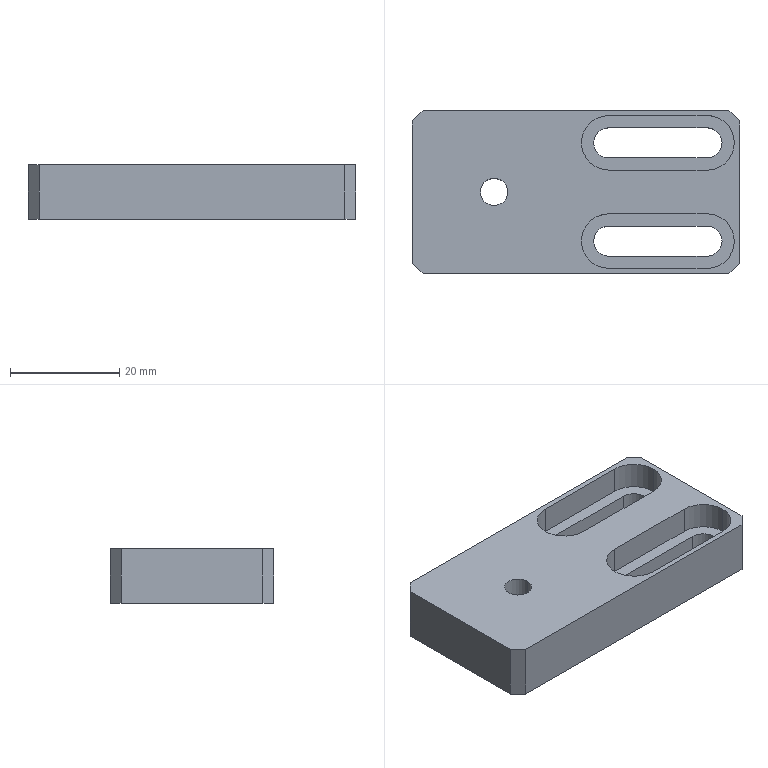Part | STEP file | 08-09 idler mounting plate | 1 solid | 34 faces | box 60 x 30 x 10 mm | volume 13911 mm3 | plane 20 | cylinder 14 | commonest cylinder face diameters 5.5 x6 10 x6 5 x2
STEP:
#1=CARTESIAN_POINT('',(29.,-9.,5.));
#2=VERTEX_POINT('',#1);
#3=CARTESIAN_POINT('',(24.,-4.,5.));
#4=VERTEX_POINT('',#3);
#5=CARTESIAN_POINT('',(24.,-9.,5.));
#6=DIRECTION('',(0.,0.,1.));
#7=DIRECTION('',(-1.,0.,0.));
#8=AXIS2_PLACEMENT_3D('',#5,#6,#7);
#9=CIRCLE('',#8,5.);
#10=EDGE_CURVE('',#2,#4,#9,.T.);
#11=ORIENTED_EDGE('',*,*,#10,.F.);
#12=CARTESIAN_POINT('',(29.,-9.,10.));
#13=VERTEX_POINT('',#12);
#14=CARTESIAN_POINT('',(29.,-9.,5.));
#15=DIRECTION('',(0.,0.,1.));
#16=VECTOR('',#15,1000.);
#17=LINE('',#14,#16);
#18=EDGE_CURVE('',#2,#13,#17,.T.);
#19=ORIENTED_EDGE('',*,*,#18,.T.);
#20=CARTESIAN_POINT('',(24.,-4.,10.));
#21=VERTEX_POINT('',#20);
#22=CARTESIAN_POINT('',(24.,-9.,10.));
#23=DIRECTION('',(0.,0.,1.));
#24=DIRECTION('',(-1.,0.,0.));
#25=AXIS2_PLACEMENT_3D('',#22,#23,#24);
#26=CIRCLE('',#25,5.);
#27=EDGE_CURVE('',#13,#21,#26,.T.);
#28=ORIENTED_EDGE('',*,*,#27,.T.);
#29=CARTESIAN_POINT('',(24.,-4.,5.));
#30=DIRECTION('',(0.,0.,1.));
#31=VECTOR('',#30,1000.);
#32=LINE('',#29,#31);
#33=EDGE_CURVE('',#4,#21,#32,.T.);
#34=ORIENTED_EDGE('',*,*,#33,.F.);
#35=EDGE_LOOP('',(#11,#19,#28,#34));
#36=FACE_OUTER_BOUND('',#35,.T.);
#37=CARTESIAN_POINT('',(24.,-9.,5.));
#38=DIRECTION('',(0.,0.,1.));
#39=DIRECTION('',(1.,0.,0.));
#40=AXIS2_PLACEMENT_3D('',#37,#38,#39);
#41=CYLINDRICAL_SURFACE('',#40,5.);
#42=ADVANCED_FACE('',(#36),#41,.F.);
#43=CARTESIAN_POINT('',(29.,9.,5.));
#44=VERTEX_POINT('',#43);
#45=CARTESIAN_POINT('',(24.,14.,5.));
#46=VERTEX_POINT('',#45);
#47=CARTESIAN_POINT('',(24.,9.,5.));
#48=DIRECTION('',(0.,0.,1.));
#49=DIRECTION('',(1.,0.,0.));
#50=AXIS2_PLACEMENT_3D('',#47,#48,#49);
#51=CIRCLE('',#50,5.);
#52=EDGE_CURVE('',#44,#46,#51,.T.);
#53=ORIENTED_EDGE('',*,*,#52,.F.);
#54=CARTESIAN_POINT('',(29.,9.,10.));
#55=VERTEX_POINT('',#54);
#56=CARTESIAN_POINT('',(29.,9.,5.));
#57=DIRECTION('',(0.,0.,1.));
#58=VECTOR('',#57,1000.);
#59=LINE('',#56,#58);
#60=EDGE_CURVE('',#44,#55,#59,.T.);
#61=ORIENTED_EDGE('',*,*,#60,.T.);
#62=CARTESIAN_POINT('',(24.,14.,10.));
#63=VERTEX_POINT('',#62);
#64=CARTESIAN_POINT('',(24.,9.,10.));
#65=DIRECTION('',(0.,0.,1.));
#66=DIRECTION('',(1.,0.,0.));
#67=AXIS2_PLACEMENT_3D('',#64,#65,#66);
#68=CIRCLE('',#67,5.);
#69=EDGE_CURVE('',#55,#63,#68,.T.);
#70=ORIENTED_EDGE('',*,*,#69,.T.);
#71=CARTESIAN_POINT('',(24.,14.,5.));
#72=DIRECTION('',(0.,0.,1.));
#73=VECTOR('',#72,1000.);
#74=LINE('',#71,#73);
#75=EDGE_CURVE('',#46,#63,#74,.T.);
#76=ORIENTED_EDGE('',*,*,#75,.F.);
#77=EDGE_LOOP('',(#53,#61,#70,#76));
#78=FACE_OUTER_BOUND('',#77,.T.);
#79=CARTESIAN_POINT('',(24.,9.,5.));
#80=DIRECTION('',(0.,0.,1.));
#81=DIRECTION('',(1.,0.,0.));
#82=AXIS2_PLACEMENT_3D('',#79,#80,#81);
#83=CYLINDRICAL_SURFACE('',#82,5.);
#84=ADVANCED_FACE('',(#78),#83,.F.);
#85=CARTESIAN_POINT('',(26.75,-9.,0.));
#86=VERTEX_POINT('',#85);
#87=CARTESIAN_POINT('',(24.,-6.25,0.));
#88=VERTEX_POINT('',#87);
#89=CARTESIAN_POINT('',(24.,-9.,0.));
#90=DIRECTION('',(0.,0.,1.));
#91=DIRECTION('',(-1.,0.,0.));
#92=AXIS2_PLACEMENT_3D('',#89,#90,#91);
#93=CIRCLE('',#92,2.75);
#94=EDGE_CURVE('',#86,#88,#93,.T.);
#95=ORIENTED_EDGE('',*,*,#94,.F.);
#96=CARTESIAN_POINT('',(26.75,-9.,5.));
#97=VERTEX_POINT('',#96);
#98=CARTESIAN_POINT('',(26.75,-9.,0.));
#99=DIRECTION('',(0.,0.,1.));
#100=VECTOR('',#99,1000.);
#101=LINE('',#98,#100);
#102=EDGE_CURVE('',#86,#97,#101,.T.);
#103=ORIENTED_EDGE('',*,*,#102,.T.);
#104=CARTESIAN_POINT('',(24.,-6.25,5.));
#105=VERTEX_POINT('',#104);
#106=CARTESIAN_POINT('',(24.,-9.,5.));
#107=DIRECTION('',(0.,0.,1.));
#108=DIRECTION('',(-1.,0.,0.));
#109=AXIS2_PLACEMENT_3D('',#106,#107,#108);
#110=CIRCLE('',#109,2.75);
#111=EDGE_CURVE('',#97,#105,#110,.T.);
#112=ORIENTED_EDGE('',*,*,#111,.T.);
#113=CARTESIAN_POINT('',(24.,-6.25,0.));
#114=DIRECTION('',(0.,0.,1.));
#115=VECTOR('',#114,1000.);
#116=LINE('',#113,#115);
#117=EDGE_CURVE('',#88,#105,#116,.T.);
#118=ORIENTED_EDGE('',*,*,#117,.F.);
#119=EDGE_LOOP('',(#95,#103,#112,#118));
#120=FACE_OUTER_BOUND('',#119,.T.);
#121=CARTESIAN_POINT('',(24.,-9.,0.));
#122=DIRECTION('',(0.,0.,1.));
#123=DIRECTION('',(1.,0.,0.));
#124=AXIS2_PLACEMENT_3D('',#121,#122,#123);
#125=CYLINDRICAL_SURFACE('',#124,2.75);
#126=ADVANCED_FACE('',(#120),#125,.F.);
#127=CARTESIAN_POINT('',(-17.5,0.,0.));
#128=VERTEX_POINT('',#127);
#129=CARTESIAN_POINT('',(-12.5,0.,0.));
#130=VERTEX_POINT('',#129);
#131=CARTESIAN_POINT('',(-15.,0.,0.));
#132=DIRECTION('',(0.,0.,1.));
#133=DIRECTION('',(1.,0.,0.));
#134=AXIS2_PLACEMENT_3D('',#131,#132,#133);
#135=CIRCLE('',#134,2.5);
#136=EDGE_CURVE('',#128,#130,#135,.T.);
#137=ORIENTED_EDGE('',*,*,#136,.F.);
#138=CARTESIAN_POINT('',(-17.5,0.,10.));
#139=VERTEX_POINT('',#138);
#140=CARTESIAN_POINT('',(-17.5,0.,10.));
#141=DIRECTION('',(0.,0.,1.));
#142=VECTOR('',#141,1000.);
#143=LINE('',#140,#142);
#144=EDGE_CURVE('',#128,#139,#143,.T.);
#145=ORIENTED_EDGE('',*,*,#144,.T.);
#146=CARTESIAN_POINT('',(-12.5,0.,10.));
#147=VERTEX_POINT('',#146);
#148=CARTESIAN_POINT('',(-15.,0.,10.));
#149=DIRECTION('',(0.,0.,1.));
#150=DIRECTION('',(1.,0.,0.));
#151=AXIS2_PLACEMENT_3D('',#148,#149,#150);
#152=CIRCLE('',#151,2.5);
#153=EDGE_CURVE('',#139,#147,#152,.T.);
#154=ORIENTED_EDGE('',*,*,#153,.T.);
#155=CARTESIAN_POINT('',(-12.5,0.,10.));
#156=DIRECTION('',(0.,0.,1.));
#157=VECTOR('',#156,1000.);
#158=LINE('',#155,#157);
#159=EDGE_CURVE('',#130,#147,#158,.T.);
#160=ORIENTED_EDGE('',*,*,#159,.F.);
#161=EDGE_LOOP('',(#137,#145,#154,#160));
#162=FACE_OUTER_BOUND('',#161,.T.);
#163=CARTESIAN_POINT('',(-15.,0.,10.));
#164=DIRECTION('',(0.,0.,1.));
#165=DIRECTION('',(1.,0.,0.));
#166=AXIS2_PLACEMENT_3D('',#163,#164,#165);
#167=CYLINDRICAL_SURFACE('',#166,2.5);
#168=ADVANCED_FACE('',(#162),#167,.F.);
#169=CARTESIAN_POINT('',(26.75,9.,0.));
#170=VERTEX_POINT('',#169);
#171=CARTESIAN_POINT('',(24.,11.75,0.));
#172=VERTEX_POINT('',#171);
#173=CARTESIAN_POINT('',(24.,9.,0.));
#174=DIRECTION('',(0.,0.,1.));
#175=DIRECTION('',(1.,0.,0.));
#176=AXIS2_PLACEMENT_3D('',#173,#174,#175);
#177=CIRCLE('',#176,2.75);
#178=EDGE_CURVE('',#170,#172,#177,.T.);
#179=ORIENTED_EDGE('',*,*,#178,.F.);
#180=CARTESIAN_POINT('',(26.75,9.,5.));
#181=VERTEX_POINT('',#180);
#182=CARTESIAN_POINT('',(26.75,9.,0.));
#183=DIRECTION('',(0.,0.,1.));
#184=VECTOR('',#183,1000.);
#185=LINE('',#182,#184);
#186=EDGE_CURVE('',#170,#181,#185,.T.);
#187=ORIENTED_EDGE('',*,*,#186,.T.);
#188=CARTESIAN_POINT('',(24.,11.75,5.));
#189=VERTEX_POINT('',#188);
#190=CARTESIAN_POINT('',(24.,9.,5.));
#191=DIRECTION('',(0.,0.,-1.));
#192=DIRECTION('',(1.,0.,0.));
#193=AXIS2_PLACEMENT_3D('',#190,#191,#192);
#194=CIRCLE('',#193,2.75);
#195=EDGE_CURVE('',#189,#181,#194,.T.);
#196=ORIENTED_EDGE('',*,*,#195,.F.);
#197=CARTESIAN_POINT('',(24.,11.75,0.));
#198=DIRECTION('',(0.,0.,1.));
#199=VECTOR('',#198,1000.);
#200=LINE('',#197,#199);
#201=EDGE_CURVE('',#172,#189,#200,.T.);
#202=ORIENTED_EDGE('',*,*,#201,.F.);
#203=EDGE_LOOP('',(#179,#187,#196,#202));
#204=FACE_OUTER_BOUND('',#203,.T.);
#205=CARTESIAN_POINT('',(24.,9.,0.));
#206=DIRECTION('',(0.,0.,1.));
#207=DIRECTION('',(1.,0.,0.));
#208=AXIS2_PLACEMENT_3D('',#205,#206,#207);
#209=CYLINDRICAL_SURFACE('',#208,2.75);
#210=ADVANCED_FACE('',(#204),#209,.F.);
#211=CARTESIAN_POINT('',(6.,6.25,5.));
#212=VERTEX_POINT('',#211);
#213=CARTESIAN_POINT('',(6.,11.75,5.));
#214=VERTEX_POINT('',#213);
#215=CARTESIAN_POINT('',(6.,9.,5.));
#216=DIRECTION('',(0.,0.,-1.));
#217=DIRECTION('',(1.,0.,0.));
#218=AXIS2_PLACEMENT_3D('',#215,#216,#217);
#219=CIRCLE('',#218,2.75);
#220=EDGE_CURVE('',#212,#214,#219,.T.);
#221=ORIENTED_EDGE('',*,*,#220,.F.);
#222=CARTESIAN_POINT('',(6.,6.25,0.));
#223=VERTEX_POINT('',#222);
#224=CARTESIAN_POINT('',(6.,6.25,0.));
#225=DIRECTION('',(0.,0.,1.));
#226=VECTOR('',#225,1000.);
#227=LINE('',#224,#226);
#228=EDGE_CURVE('',#223,#212,#227,.T.);
#229=ORIENTED_EDGE('',*,*,#228,.F.);
#230=CARTESIAN_POINT('',(6.,11.75,0.));
#231=VERTEX_POINT('',#230);
#232=CARTESIAN_POINT('',(6.,9.,0.));
#233=DIRECTION('',(0.,0.,1.));
#234=DIRECTION('',(1.,0.,0.));
#235=AXIS2_PLACEMENT_3D('',#232,#233,#234);
#236=CIRCLE('',#235,2.75);
#237=EDGE_CURVE('',#231,#223,#236,.T.);
#238=ORIENTED_EDGE('',*,*,#237,.F.);
#239=CARTESIAN_POINT('',(6.,11.75,0.));
#240=DIRECTION('',(0.,0.,1.));
#241=VECTOR('',#240,1000.);
#242=LINE('',#239,#241);
#243=EDGE_CURVE('',#231,#214,#242,.T.);
#244=ORIENTED_EDGE('',*,*,#243,.T.);
#245=EDGE_LOOP('',(#221,#229,#238,#244));
#246=FACE_OUTER_BOUND('',#245,.T.);
#247=CARTESIAN_POINT('',(6.,9.,0.));
#248=DIRECTION('',(0.,0.,1.));
#249=DIRECTION('',(1.,0.,0.));
#250=AXIS2_PLACEMENT_3D('',#247,#248,#249);
#251=CYLINDRICAL_SURFACE('',#250,2.75);
#252=ADVANCED_FACE('',(#246),#251,.F.);
#253=CARTESIAN_POINT('',(6.,11.75,5.));
#254=DIRECTION('',(1.,0.,0.));
#255=VECTOR('',#254,1000.);
#256=LINE('',#253,#255);
#257=EDGE_CURVE('',#214,#189,#256,.T.);
#258=ORIENTED_EDGE('',*,*,#257,.F.);
#259=ORIENTED_EDGE('',*,*,#243,.F.);
#260=CARTESIAN_POINT('',(6.,11.75,0.));
#261=DIRECTION('',(-1.,0.,0.));
#262=VECTOR('',#261,1000.);
#263=LINE('',#260,#262);
#264=EDGE_CURVE('',#172,#231,#263,.T.);
#265=ORIENTED_EDGE('',*,*,#264,.F.);
#266=ORIENTED_EDGE('',*,*,#201,.T.);
#267=EDGE_LOOP('',(#258,#259,#265,#266));
#268=FACE_OUTER_BOUND('',#267,.T.);
#269=CARTESIAN_POINT('',(6.,11.75,0.));
#270=DIRECTION('',(0.,1.,0.));
#271=DIRECTION('',(0.,0.,1.));
#272=AXIS2_PLACEMENT_3D('',#269,#270,#271);
#273=PLANE('',#272);
#274=ADVANCED_FACE('',(#268),#273,.F.);
#275=ORIENTED_EDGE('',*,*,#186,.F.);
#276=CARTESIAN_POINT('',(24.,6.25,0.));
#277=VERTEX_POINT('',#276);
#278=CARTESIAN_POINT('',(24.,9.,0.));
#279=DIRECTION('',(0.,0.,1.));
#280=DIRECTION('',(1.,0.,0.));
#281=AXIS2_PLACEMENT_3D('',#278,#279,#280);
#282=CIRCLE('',#281,2.75);
#283=EDGE_CURVE('',#277,#170,#282,.T.);
#284=ORIENTED_EDGE('',*,*,#283,.F.);
#285=CARTESIAN_POINT('',(24.,6.25,5.));
#286=VERTEX_POINT('',#285);
#287=CARTESIAN_POINT('',(24.,6.25,0.));
#288=DIRECTION('',(0.,0.,1.));
#289=VECTOR('',#288,1000.);
#290=LINE('',#287,#289);
#291=EDGE_CURVE('',#277,#286,#290,.T.);
#292=ORIENTED_EDGE('',*,*,#291,.T.);
#293=CARTESIAN_POINT('',(24.,9.,5.));
#294=DIRECTION('',(0.,0.,-1.));
#295=DIRECTION('',(1.,0.,0.));
#296=AXIS2_PLACEMENT_3D('',#293,#294,#295);
#297=CIRCLE('',#296,2.75);
#298=EDGE_CURVE('',#181,#286,#297,.T.);
#299=ORIENTED_EDGE('',*,*,#298,.F.);
#300=EDGE_LOOP('',(#275,#284,#292,#299));
#301=FACE_OUTER_BOUND('',#300,.T.);
#302=CARTESIAN_POINT('',(24.,9.,0.));
#303=DIRECTION('',(0.,0.,1.));
#304=DIRECTION('',(1.,0.,0.));
#305=AXIS2_PLACEMENT_3D('',#302,#303,#304);
#306=CYLINDRICAL_SURFACE('',#305,2.75);
#307=ADVANCED_FACE('',(#301),#306,.F.);
#308=CARTESIAN_POINT('',(6.,6.25,5.));
#309=DIRECTION('',(-1.,0.,0.));
#310=VECTOR('',#309,1000.);
#311=LINE('',#308,#310);
#312=EDGE_CURVE('',#286,#212,#311,.T.);
#313=ORIENTED_EDGE('',*,*,#312,.F.);
#314=ORIENTED_EDGE('',*,*,#291,.F.);
#315=CARTESIAN_POINT('',(6.,6.25,0.));
#316=DIRECTION('',(1.,0.,0.));
#317=VECTOR('',#316,1000.);
#318=LINE('',#315,#317);
#319=EDGE_CURVE('',#223,#277,#318,.T.);
#320=ORIENTED_EDGE('',*,*,#319,.F.);
#321=ORIENTED_EDGE('',*,*,#228,.T.);
#322=EDGE_LOOP('',(#313,#314,#320,#321));
#323=FACE_OUTER_BOUND('',#322,.T.);
#324=CARTESIAN_POINT('',(6.,6.25,0.));
#325=DIRECTION('',(0.,-1.,0.));
#326=DIRECTION('',(0.,0.,-1.));
#327=AXIS2_PLACEMENT_3D('',#324,#325,#326);
#328=PLANE('',#327);
#329=ADVANCED_FACE('',(#323),#328,.F.);
#330=CARTESIAN_POINT('',(30.,-13.,10.));
#331=VERTEX_POINT('',#330);
#332=CARTESIAN_POINT('',(30.,13.,10.));
#333=VERTEX_POINT('',#332);
#334=CARTESIAN_POINT('',(30.,15.,10.));
#335=DIRECTION('',(0.,1.,0.));
#336=VECTOR('',#335,1000.);
#337=LINE('',#334,#336);
#338=EDGE_CURVE('',#331,#333,#337,.T.);
#339=ORIENTED_EDGE('',*,*,#338,.F.);
#340=CARTESIAN_POINT('',(30.,-13.,0.));
#341=VERTEX_POINT('',#340);
#342=CARTESIAN_POINT('',(30.,-13.,10.));
#343=DIRECTION('',(0.,0.,-1.));
#344=VECTOR('',#343,1000.);
#345=LINE('',#342,#344);
#346=EDGE_CURVE('',#331,#341,#345,.T.);
#347=ORIENTED_EDGE('',*,*,#346,.T.);
#348=CARTESIAN_POINT('',(30.,13.,0.));
#349=VERTEX_POINT('',#348);
#350=CARTESIAN_POINT('',(30.,15.,0.));
#351=DIRECTION('',(0.,1.,0.));
#352=VECTOR('',#351,1000.);
#353=LINE('',#350,#352);
#354=EDGE_CURVE('',#341,#349,#353,.T.);
#355=ORIENTED_EDGE('',*,*,#354,.T.);
#356=CARTESIAN_POINT('',(30.,13.,10.));
#357=DIRECTION('',(0.,0.,1.));
#358=VECTOR('',#357,1000.);
#359=LINE('',#356,#358);
#360=EDGE_CURVE('',#349,#333,#359,.T.);
#361=ORIENTED_EDGE('',*,*,#360,.T.);
#362=EDGE_LOOP('',(#339,#347,#355,#361));
#363=FACE_OUTER_BOUND('',#362,.T.);
#364=CARTESIAN_POINT('',(30.,15.,10.));
#365=DIRECTION('',(-1.,0.,0.));
#366=DIRECTION('',(0.,-1.,0.));
#367=AXIS2_PLACEMENT_3D('',#364,#365,#366);
#368=PLANE('',#367);
#369=ADVANCED_FACE('',(#363),#368,.F.);
#370=CARTESIAN_POINT('',(28.,15.,10.));
#371=VERTEX_POINT('',#370);
#372=CARTESIAN_POINT('',(-28.,15.,10.));
#373=VERTEX_POINT('',#372);
#374=CARTESIAN_POINT('',(-30.,15.,10.));
#375=DIRECTION('',(-1.,0.,0.));
#376=VECTOR('',#375,1000.);
#377=LINE('',#374,#376);
#378=EDGE_CURVE('',#371,#373,#377,.T.);
#379=ORIENTED_EDGE('',*,*,#378,.F.);
#380=CARTESIAN_POINT('',(28.,15.,0.));
#381=VERTEX_POINT('',#380);
#382=CARTESIAN_POINT('',(28.,15.,10.));
#383=DIRECTION('',(0.,0.,-1.));
#384=VECTOR('',#383,1000.);
#385=LINE('',#382,#384);
#386=EDGE_CURVE('',#371,#381,#385,.T.);
#387=ORIENTED_EDGE('',*,*,#386,.T.);
#388=CARTESIAN_POINT('',(-28.,15.,0.));
#389=VERTEX_POINT('',#388);
#390=CARTESIAN_POINT('',(-30.,15.,0.));
#391=DIRECTION('',(-1.,0.,0.));
#392=VECTOR('',#391,1000.);
#393=LINE('',#390,#392);
#394=EDGE_CURVE('',#381,#389,#393,.T.);
#395=ORIENTED_EDGE('',*,*,#394,.T.);
#396=CARTESIAN_POINT('',(-28.,15.,10.));
#397=DIRECTION('',(0.,0.,1.));
#398=VECTOR('',#397,1000.);
#399=LINE('',#396,#398);
#400=EDGE_CURVE('',#389,#373,#399,.T.);
#401=ORIENTED_EDGE('',*,*,#400,.T.);
#402=EDGE_LOOP('',(#379,#387,#395,#401));
#403=FACE_OUTER_BOUND('',#402,.T.);
#404=CARTESIAN_POINT('',(-30.,15.,10.));
#405=DIRECTION('',(0.,-1.,0.));
#406=DIRECTION('',(0.,0.,-1.));
#407=AXIS2_PLACEMENT_3D('',#404,#405,#406);
#408=PLANE('',#407);
#409=ADVANCED_FACE('',(#403),#408,.F.);
#410=CARTESIAN_POINT('',(-30.,13.,0.));
#411=VERTEX_POINT('',#410);
#412=CARTESIAN_POINT('',(-30.,-13.,0.));
#413=VERTEX_POINT('',#412);
#414=CARTESIAN_POINT('',(-30.,15.,0.));
#415=DIRECTION('',(0.,-1.,0.));
#416=VECTOR('',#415,1000.);
#417=LINE('',#414,#416);
#418=EDGE_CURVE('',#411,#413,#417,.T.);
#419=ORIENTED_EDGE('',*,*,#418,.T.);
#420=CARTESIAN_POINT('',(-30.,-13.,10.));
#421=VERTEX_POINT('',#420);
#422=CARTESIAN_POINT('',(-30.,-13.,10.));
#423=DIRECTION('',(0.,0.,1.));
#424=VECTOR('',#423,1000.);
#425=LINE('',#422,#424);
#426=EDGE_CURVE('',#413,#421,#425,.T.);
#427=ORIENTED_EDGE('',*,*,#426,.T.);
#428=CARTESIAN_POINT('',(-30.,13.,10.));
#429=VERTEX_POINT('',#428);
#430=CARTESIAN_POINT('',(-30.,15.,10.));
#431=DIRECTION('',(0.,-1.,0.));
#432=VECTOR('',#431,1000.);
#433=LINE('',#430,#432);
#434=EDGE_CURVE('',#429,#421,#433,.T.);
#435=ORIENTED_EDGE('',*,*,#434,.F.);
#436=CARTESIAN_POINT('',(-30.,13.,10.));
#437=DIRECTION('',(0.,0.,-1.));
#438=VECTOR('',#437,1000.);
#439=LINE('',#436,#438);
#440=EDGE_CURVE('',#429,#411,#439,.T.);
#441=ORIENTED_EDGE('',*,*,#440,.T.);
#442=EDGE_LOOP('',(#419,#427,#435,#441));
#443=FACE_OUTER_BOUND('',#442,.T.);
#444=CARTESIAN_POINT('',(-30.,15.,10.));
#445=DIRECTION('',(1.,0.,0.));
#446=DIRECTION('',(0.,1.,0.));
#447=AXIS2_PLACEMENT_3D('',#444,#445,#446);
#448=PLANE('',#447);
#449=ADVANCED_FACE('',(#443),#448,.F.);
#450=CARTESIAN_POINT('',(-28.,-15.,0.));
#451=VERTEX_POINT('',#450);
#452=CARTESIAN_POINT('',(28.,-15.,0.));
#453=VERTEX_POINT('',#452);
#454=CARTESIAN_POINT('',(-30.,-15.,0.));
#455=DIRECTION('',(1.,0.,0.));
#456=VECTOR('',#455,1000.);
#457=LINE('',#454,#456);
#458=EDGE_CURVE('',#451,#453,#457,.T.);
#459=ORIENTED_EDGE('',*,*,#458,.T.);
#460=CARTESIAN_POINT('',(28.,-15.,10.));
#461=VERTEX_POINT('',#460);
#462=CARTESIAN_POINT('',(28.,-15.,10.));
#463=DIRECTION('',(0.,0.,1.));
#464=VECTOR('',#463,1000.);
#465=LINE('',#462,#464);
#466=EDGE_CURVE('',#453,#461,#465,.T.);
#467=ORIENTED_EDGE('',*,*,#466,.T.);
#468=CARTESIAN_POINT('',(-28.,-15.,10.));
#469=VERTEX_POINT('',#468);
#470=CARTESIAN_POINT('',(-30.,-15.,10.));
#471=DIRECTION('',(1.,0.,0.));
#472=VECTOR('',#471,1000.);
#473=LINE('',#470,#472);
#474=EDGE_CURVE('',#469,#461,#473,.T.);
#475=ORIENTED_EDGE('',*,*,#474,.F.);
#476=CARTESIAN_POINT('',(-28.,-15.,10.));
#477=DIRECTION('',(0.,0.,-1.));
#478=VECTOR('',#477,1000.);
#479=LINE('',#476,#478);
#480=EDGE_CURVE('',#469,#451,#479,.T.);
#481=ORIENTED_EDGE('',*,*,#480,.T.);
#482=EDGE_LOOP('',(#459,#467,#475,#481));
#483=FACE_OUTER_BOUND('',#482,.T.);
#484=CARTESIAN_POINT('',(-30.,-15.,10.));
#485=DIRECTION('',(0.,1.,0.));
#486=DIRECTION('',(0.,0.,1.));
#487=AXIS2_PLACEMENT_3D('',#484,#485,#486);
#488=PLANE('',#487);
#489=ADVANCED_FACE('',(#483),#488,.F.);
#490=CARTESIAN_POINT('',(6.,-4.,10.));
#491=VERTEX_POINT('',#490);
#492=CARTESIAN_POINT('',(6.,-14.,10.));
#493=VERTEX_POINT('',#492);
#494=CARTESIAN_POINT('',(6.,-9.,10.));
#495=DIRECTION('',(0.,0.,1.));
#496=DIRECTION('',(-1.,0.,0.));
#497=AXIS2_PLACEMENT_3D('',#494,#495,#496);
#498=CIRCLE('',#497,5.);
#499=EDGE_CURVE('',#491,#493,#498,.T.);
#500=ORIENTED_EDGE('',*,*,#499,.F.);
#501=CARTESIAN_POINT('',(6.,-4.,10.));
#502=DIRECTION('',(-1.,0.,0.));
#503=VECTOR('',#502,1000.);
#504=LINE('',#501,#503);
#505=EDGE_CURVE('',#21,#491,#504,.T.);
#506=ORIENTED_EDGE('',*,*,#505,.F.);
#507=ORIENTED_EDGE('',*,*,#27,.F.);
#508=CARTESIAN_POINT('',(24.,-14.,10.));
#509=VERTEX_POINT('',#508);
#510=CARTESIAN_POINT('',(24.,-9.,10.));
#511=DIRECTION('',(0.,0.,1.));
#512=DIRECTION('',(-1.,0.,0.));
#513=AXIS2_PLACEMENT_3D('',#510,#511,#512);
#514=CIRCLE('',#513,5.);
#515=EDGE_CURVE('',#509,#13,#514,.T.);
#516=ORIENTED_EDGE('',*,*,#515,.F.);
#517=CARTESIAN_POINT('',(6.,-14.,10.));
#518=DIRECTION('',(1.,0.,0.));
#519=VECTOR('',#518,1000.);
#520=LINE('',#517,#519);
#521=EDGE_CURVE('',#493,#509,#520,.T.);
#522=ORIENTED_EDGE('',*,*,#521,.F.);
#523=EDGE_LOOP('',(#500,#506,#507,#516,#522));
#524=FACE_BOUND('',#523,.T.);
#525=CARTESIAN_POINT('',(6.,14.,10.));
#526=VERTEX_POINT('',#525);
#527=CARTESIAN_POINT('',(6.,4.,10.));
#528=VERTEX_POINT('',#527);
#529=CARTESIAN_POINT('',(6.,9.,10.));
#530=DIRECTION('',(0.,0.,1.));
#531=DIRECTION('',(1.,0.,0.));
#532=AXIS2_PLACEMENT_3D('',#529,#530,#531);
#533=CIRCLE('',#532,5.);
#534=EDGE_CURVE('',#526,#528,#533,.T.);
#535=ORIENTED_EDGE('',*,*,#534,.F.);
#536=CARTESIAN_POINT('',(6.,14.,10.));
#537=DIRECTION('',(-1.,0.,0.));
#538=VECTOR('',#537,1000.);
#539=LINE('',#536,#538);
#540=EDGE_CURVE('',#63,#526,#539,.T.);
#541=ORIENTED_EDGE('',*,*,#540,.F.);
#542=ORIENTED_EDGE('',*,*,#69,.F.);
#543=CARTESIAN_POINT('',(24.,4.,10.));
#544=VERTEX_POINT('',#543);
#545=CARTESIAN_POINT('',(24.,9.,10.));
#546=DIRECTION('',(0.,0.,1.));
#547=DIRECTION('',(1.,0.,0.));
#548=AXIS2_PLACEMENT_3D('',#545,#546,#547);
#549=CIRCLE('',#548,5.);
#550=EDGE_CURVE('',#544,#55,#549,.T.);
#551=ORIENTED_EDGE('',*,*,#550,.F.);
#552=CARTESIAN_POINT('',(6.,4.,10.));
#553=DIRECTION('',(1.,0.,0.));
#554=VECTOR('',#553,1000.);
#555=LINE('',#552,#554);
#556=EDGE_CURVE('',#528,#544,#555,.T.);
#557=ORIENTED_EDGE('',*,*,#556,.F.);
#558=EDGE_LOOP('',(#535,#541,#542,#551,#557));
#559=FACE_BOUND('',#558,.T.);
#560=CARTESIAN_POINT('',(-15.,0.,10.));
#561=DIRECTION('',(0.,0.,1.));
#562=DIRECTION('',(1.,0.,0.));
#563=AXIS2_PLACEMENT_3D('',#560,#561,#562);
#564=CIRCLE('',#563,2.5);
#565=EDGE_CURVE('',#147,#139,#564,.T.);
#566=ORIENTED_EDGE('',*,*,#565,.F.);
#567=ORIENTED_EDGE('',*,*,#153,.F.);
#568=EDGE_LOOP('',(#566,#567));
#569=FACE_BOUND('',#568,.T.);
#570=ORIENTED_EDGE('',*,*,#474,.T.);
#571=CARTESIAN_POINT('',(29.,-14.,10.));
#572=DIRECTION('',(0.7071,0.7071,0.));
#573=VECTOR('',#572,1000.);
#574=LINE('',#571,#573);
#575=EDGE_CURVE('',#461,#331,#574,.T.);
#576=ORIENTED_EDGE('',*,*,#575,.T.);
#577=ORIENTED_EDGE('',*,*,#338,.T.);
#578=CARTESIAN_POINT('',(44.,-1.,10.));
#579=DIRECTION('',(-0.7071,0.7071,0.));
#580=VECTOR('',#579,1000.);
#581=LINE('',#578,#580);
#582=EDGE_CURVE('',#333,#371,#581,.T.);
#583=ORIENTED_EDGE('',*,*,#582,.T.);
#584=ORIENTED_EDGE('',*,*,#378,.T.);
#585=CARTESIAN_POINT('',(-14.,29.,10.));
#586=DIRECTION('',(-0.7071,-0.7071,0.));
#587=VECTOR('',#586,1000.);
#588=LINE('',#585,#587);
#589=EDGE_CURVE('',#373,#429,#588,.T.);
#590=ORIENTED_EDGE('',*,*,#589,.T.);
#591=ORIENTED_EDGE('',*,*,#434,.T.);
#592=CARTESIAN_POINT('',(1.,-44.,10.));
#593=DIRECTION('',(0.7071,-0.7071,0.));
#594=VECTOR('',#593,1000.);
#595=LINE('',#592,#594);
#596=EDGE_CURVE('',#421,#469,#595,.T.);
#597=ORIENTED_EDGE('',*,*,#596,.T.);
#598=EDGE_LOOP('',(#570,#576,#577,#583,#584,#590,#591,#597));
#599=FACE_OUTER_BOUND('',#598,.T.);
#600=CARTESIAN_POINT('',(30.,-15.,10.));
#601=DIRECTION('',(0.,0.,1.));
#602=DIRECTION('',(1.,0.,0.));
#603=AXIS2_PLACEMENT_3D('',#600,#601,#602);
#604=PLANE('',#603);
#605=ADVANCED_FACE('',(#524,#559,#569,#599),#604,.T.);
#606=CARTESIAN_POINT('',(6.,-6.25,0.));
#607=VERTEX_POINT('',#606);
#608=CARTESIAN_POINT('',(6.,-6.25,0.));
#609=DIRECTION('',(-1.,0.,0.));
#610=VECTOR('',#609,1000.);
#611=LINE('',#608,#610);
#612=EDGE_CURVE('',#88,#607,#611,.T.);
#613=ORIENTED_EDGE('',*,*,#612,.T.);
#614=CARTESIAN_POINT('',(6.,-11.75,0.));
#615=VERTEX_POINT('',#614);
#616=CARTESIAN_POINT('',(6.,-9.,0.));
#617=DIRECTION('',(0.,0.,1.));
#618=DIRECTION('',(-1.,0.,0.));
#619=AXIS2_PLACEMENT_3D('',#616,#617,#618);
#620=CIRCLE('',#619,2.75);
#621=EDGE_CURVE('',#607,#615,#620,.T.);
#622=ORIENTED_EDGE('',*,*,#621,.T.);
#623=CARTESIAN_POINT('',(24.,-11.75,0.));
#624=VERTEX_POINT('',#623);
#625=CARTESIAN_POINT('',(6.,-11.75,0.));
#626=DIRECTION('',(1.,0.,0.));
#627=VECTOR('',#626,1000.);
#628=LINE('',#625,#627);
#629=EDGE_CURVE('',#615,#624,#628,.T.);
#630=ORIENTED_EDGE('',*,*,#629,.T.);
#631=CARTESIAN_POINT('',(24.,-9.,0.));
#632=DIRECTION('',(0.,0.,1.));
#633=DIRECTION('',(-1.,0.,0.));
#634=AXIS2_PLACEMENT_3D('',#631,#632,#633);
#635=CIRCLE('',#634,2.75);
#636=EDGE_CURVE('',#624,#86,#635,.T.);
#637=ORIENTED_EDGE('',*,*,#636,.T.);
#638=ORIENTED_EDGE('',*,*,#94,.T.);
#639=EDGE_LOOP('',(#613,#622,#630,#637,#638));
#640=FACE_BOUND('',#639,.T.);
#641=ORIENTED_EDGE('',*,*,#264,.T.);
#642=ORIENTED_EDGE('',*,*,#237,.T.);
#643=ORIENTED_EDGE('',*,*,#319,.T.);
#644=ORIENTED_EDGE('',*,*,#283,.T.);
#645=ORIENTED_EDGE('',*,*,#178,.T.);
#646=EDGE_LOOP('',(#641,#642,#643,#644,#645));
#647=FACE_BOUND('',#646,.T.);
#648=CARTESIAN_POINT('',(-15.,0.,0.));
#649=DIRECTION('',(0.,0.,1.));
#650=DIRECTION('',(1.,0.,0.));
#651=AXIS2_PLACEMENT_3D('',#648,#649,#650);
#652=CIRCLE('',#651,2.5);
#653=EDGE_CURVE('',#130,#128,#652,.T.);
#654=ORIENTED_EDGE('',*,*,#653,.T.);
#655=ORIENTED_EDGE('',*,*,#136,.T.);
#656=EDGE_LOOP('',(#654,#655));
#657=FACE_BOUND('',#656,.T.);
#658=ORIENTED_EDGE('',*,*,#354,.F.);
#659=CARTESIAN_POINT('',(30.,-13.,0.));
#660=DIRECTION('',(-0.7071,-0.7071,0.));
#661=VECTOR('',#660,1000.);
#662=LINE('',#659,#661);
#663=EDGE_CURVE('',#341,#453,#662,.T.);
#664=ORIENTED_EDGE('',*,*,#663,.T.);
#665=ORIENTED_EDGE('',*,*,#458,.F.);
#666=CARTESIAN_POINT('',(-28.,-15.,0.));
#667=DIRECTION('',(-0.7071,0.7071,0.));
#668=VECTOR('',#667,1000.);
#669=LINE('',#666,#668);
#670=EDGE_CURVE('',#451,#413,#669,.T.);
#671=ORIENTED_EDGE('',*,*,#670,.T.);
#672=ORIENTED_EDGE('',*,*,#418,.F.);
#673=CARTESIAN_POINT('',(-30.,13.,0.));
#674=DIRECTION('',(0.7071,0.7071,0.));
#675=VECTOR('',#674,1000.);
#676=LINE('',#673,#675);
#677=EDGE_CURVE('',#411,#389,#676,.T.);
#678=ORIENTED_EDGE('',*,*,#677,.T.);
#679=ORIENTED_EDGE('',*,*,#394,.F.);
#680=CARTESIAN_POINT('',(28.,15.,0.));
#681=DIRECTION('',(0.7071,-0.7071,0.));
#682=VECTOR('',#681,1000.);
#683=LINE('',#680,#682);
#684=EDGE_CURVE('',#381,#349,#683,.T.);
#685=ORIENTED_EDGE('',*,*,#684,.T.);
#686=EDGE_LOOP('',(#658,#664,#665,#671,#672,#678,#679,#685));
#687=FACE_OUTER_BOUND('',#686,.T.);
#688=CARTESIAN_POINT('',(30.,-15.,0.));
#689=DIRECTION('',(0.,0.,1.));
#690=DIRECTION('',(1.,0.,0.));
#691=AXIS2_PLACEMENT_3D('',#688,#689,#690);
#692=PLANE('',#691);
#693=ADVANCED_FACE('',(#640,#647,#657,#687),#692,.F.);
#694=ORIENTED_EDGE('',*,*,#144,.F.);
#695=ORIENTED_EDGE('',*,*,#653,.F.);
#696=ORIENTED_EDGE('',*,*,#159,.T.);
#697=ORIENTED_EDGE('',*,*,#565,.T.);
#698=EDGE_LOOP('',(#694,#695,#696,#697));
#699=FACE_OUTER_BOUND('',#698,.T.);
#700=CARTESIAN_POINT('',(-15.,0.,10.));
#701=DIRECTION('',(0.,0.,1.));
#702=DIRECTION('',(1.,0.,0.));
#703=AXIS2_PLACEMENT_3D('',#700,#701,#702);
#704=CYLINDRICAL_SURFACE('',#703,2.5);
#705=ADVANCED_FACE('',(#699),#704,.F.);
#706=ORIENTED_EDGE('',*,*,#575,.F.);
#707=ORIENTED_EDGE('',*,*,#466,.F.);
#708=ORIENTED_EDGE('',*,*,#663,.F.);
#709=ORIENTED_EDGE('',*,*,#346,.F.);
#710=EDGE_LOOP('',(#706,#707,#708,#709));
#711=FACE_OUTER_BOUND('',#710,.T.);
#712=CARTESIAN_POINT('',(30.,-13.,10.));
#713=DIRECTION('',(-0.7071,0.7071,0.));
#714=DIRECTION('',(-0.7071,-0.7071,0.));
#715=AXIS2_PLACEMENT_3D('',#712,#713,#714);
#716=PLANE('',#715);
#717=ADVANCED_FACE('',(#711),#716,.F.);
#718=ORIENTED_EDGE('',*,*,#582,.F.);
#719=ORIENTED_EDGE('',*,*,#360,.F.);
#720=ORIENTED_EDGE('',*,*,#684,.F.);
#721=ORIENTED_EDGE('',*,*,#386,.F.);
#722=EDGE_LOOP('',(#718,#719,#720,#721));
#723=FACE_OUTER_BOUND('',#722,.T.);
#724=CARTESIAN_POINT('',(28.,15.,10.));
#725=DIRECTION('',(-0.7071,-0.7071,0.));
#726=DIRECTION('',(0.7071,-0.7071,0.));
#727=AXIS2_PLACEMENT_3D('',#724,#725,#726);
#728=PLANE('',#727);
#729=ADVANCED_FACE('',(#723),#728,.F.);
#730=ORIENTED_EDGE('',*,*,#596,.F.);
#731=ORIENTED_EDGE('',*,*,#426,.F.);
#732=ORIENTED_EDGE('',*,*,#670,.F.);
#733=ORIENTED_EDGE('',*,*,#480,.F.);
#734=EDGE_LOOP('',(#730,#731,#732,#733));
#735=FACE_OUTER_BOUND('',#734,.T.);
#736=CARTESIAN_POINT('',(-28.,-15.,10.));
#737=DIRECTION('',(0.7071,0.7071,0.));
#738=DIRECTION('',(-0.7071,0.7071,0.));
#739=AXIS2_PLACEMENT_3D('',#736,#737,#738);
#740=PLANE('',#739);
#741=ADVANCED_FACE('',(#735),#740,.F.);
#742=ORIENTED_EDGE('',*,*,#589,.F.);
#743=ORIENTED_EDGE('',*,*,#400,.F.);
#744=ORIENTED_EDGE('',*,*,#677,.F.);
#745=ORIENTED_EDGE('',*,*,#440,.F.);
#746=EDGE_LOOP('',(#742,#743,#744,#745));
#747=FACE_OUTER_BOUND('',#746,.T.);
#748=CARTESIAN_POINT('',(-30.,13.,10.));
#749=DIRECTION('',(0.7071,-0.7071,0.));
#750=DIRECTION('',(0.7071,0.7071,0.));
#751=AXIS2_PLACEMENT_3D('',#748,#749,#750);
#752=PLANE('',#751);
#753=ADVANCED_FACE('',(#747),#752,.F.);
#754=CARTESIAN_POINT('',(6.,-6.25,5.));
#755=VERTEX_POINT('',#754);
#756=CARTESIAN_POINT('',(6.,-6.25,0.));
#757=DIRECTION('',(0.,0.,1.));
#758=VECTOR('',#757,1000.);
#759=LINE('',#756,#758);
#760=EDGE_CURVE('',#607,#755,#759,.T.);
#761=ORIENTED_EDGE('',*,*,#760,.T.);
#762=CARTESIAN_POINT('',(6.,-11.75,5.));
#763=VERTEX_POINT('',#762);
#764=CARTESIAN_POINT('',(6.,-9.,5.));
#765=DIRECTION('',(0.,0.,1.));
#766=DIRECTION('',(-1.,0.,0.));
#767=AXIS2_PLACEMENT_3D('',#764,#765,#766);
#768=CIRCLE('',#767,2.75);
#769=EDGE_CURVE('',#755,#763,#768,.T.);
#770=ORIENTED_EDGE('',*,*,#769,.T.);
#771=CARTESIAN_POINT('',(6.,-11.75,0.));
#772=DIRECTION('',(0.,0.,1.));
#773=VECTOR('',#772,1000.);
#774=LINE('',#771,#773);
#775=EDGE_CURVE('',#615,#763,#774,.T.);
#776=ORIENTED_EDGE('',*,*,#775,.F.);
#777=ORIENTED_EDGE('',*,*,#621,.F.);
#778=EDGE_LOOP('',(#761,#770,#776,#777));
#779=FACE_OUTER_BOUND('',#778,.T.);
#780=CARTESIAN_POINT('',(6.,-9.,0.));
#781=DIRECTION('',(0.,0.,1.));
#782=DIRECTION('',(1.,0.,0.));
#783=AXIS2_PLACEMENT_3D('',#780,#781,#782);
#784=CYLINDRICAL_SURFACE('',#783,2.75);
#785=ADVANCED_FACE('',(#779),#784,.F.);
#786=ORIENTED_EDGE('',*,*,#117,.T.);
#787=CARTESIAN_POINT('',(6.,-6.25,5.));
#788=DIRECTION('',(-1.,0.,0.));
#789=VECTOR('',#788,1000.);
#790=LINE('',#787,#789);
#791=EDGE_CURVE('',#105,#755,#790,.T.);
#792=ORIENTED_EDGE('',*,*,#791,.T.);
#793=ORIENTED_EDGE('',*,*,#760,.F.);
#794=ORIENTED_EDGE('',*,*,#612,.F.);
#795=EDGE_LOOP('',(#786,#792,#793,#794));
#796=FACE_OUTER_BOUND('',#795,.T.);
#797=CARTESIAN_POINT('',(6.,-6.25,0.));
#798=DIRECTION('',(0.,1.,0.));
#799=DIRECTION('',(0.,0.,1.));
#800=AXIS2_PLACEMENT_3D('',#797,#798,#799);
#801=PLANE('',#800);
#802=ADVANCED_FACE('',(#796),#801,.F.);
#803=ORIENTED_EDGE('',*,*,#102,.F.);
#804=ORIENTED_EDGE('',*,*,#636,.F.);
#805=CARTESIAN_POINT('',(24.,-11.75,5.));
#806=VERTEX_POINT('',#805);
#807=CARTESIAN_POINT('',(24.,-11.75,0.));
#808=DIRECTION('',(0.,0.,1.));
#809=VECTOR('',#808,1000.);
#810=LINE('',#807,#809);
#811=EDGE_CURVE('',#624,#806,#810,.T.);
#812=ORIENTED_EDGE('',*,*,#811,.T.);
#813=CARTESIAN_POINT('',(24.,-9.,5.));
#814=DIRECTION('',(0.,0.,1.));
#815=DIRECTION('',(-1.,0.,0.));
#816=AXIS2_PLACEMENT_3D('',#813,#814,#815);
#817=CIRCLE('',#816,2.75);
#818=EDGE_CURVE('',#806,#97,#817,.T.);
#819=ORIENTED_EDGE('',*,*,#818,.T.);
#820=EDGE_LOOP('',(#803,#804,#812,#819));
#821=FACE_OUTER_BOUND('',#820,.T.);
#822=CARTESIAN_POINT('',(24.,-9.,0.));
#823=DIRECTION('',(0.,0.,1.));
#824=DIRECTION('',(1.,0.,0.));
#825=AXIS2_PLACEMENT_3D('',#822,#823,#824);
#826=CYLINDRICAL_SURFACE('',#825,2.75);
#827=ADVANCED_FACE('',(#821),#826,.F.);
#828=ORIENTED_EDGE('',*,*,#775,.T.);
#829=CARTESIAN_POINT('',(6.,-11.75,5.));
#830=DIRECTION('',(1.,0.,0.));
#831=VECTOR('',#830,1000.);
#832=LINE('',#829,#831);
#833=EDGE_CURVE('',#763,#806,#832,.T.);
#834=ORIENTED_EDGE('',*,*,#833,.T.);
#835=ORIENTED_EDGE('',*,*,#811,.F.);
#836=ORIENTED_EDGE('',*,*,#629,.F.);
#837=EDGE_LOOP('',(#828,#834,#835,#836));
#838=FACE_OUTER_BOUND('',#837,.T.);
#839=CARTESIAN_POINT('',(6.,-11.75,0.));
#840=DIRECTION('',(0.,-1.,0.));
#841=DIRECTION('',(0.,0.,-1.));
#842=AXIS2_PLACEMENT_3D('',#839,#840,#841);
#843=PLANE('',#842);
#844=ADVANCED_FACE('',(#838),#843,.F.);
#845=CARTESIAN_POINT('',(6.,14.,5.));
#846=VERTEX_POINT('',#845);
#847=CARTESIAN_POINT('',(6.,4.,5.));
#848=VERTEX_POINT('',#847);
#849=CARTESIAN_POINT('',(6.,9.,5.));
#850=DIRECTION('',(0.,0.,1.));
#851=DIRECTION('',(1.,0.,0.));
#852=AXIS2_PLACEMENT_3D('',#849,#850,#851);
#853=CIRCLE('',#852,5.);
#854=EDGE_CURVE('',#846,#848,#853,.T.);
#855=ORIENTED_EDGE('',*,*,#854,.T.);
#856=CARTESIAN_POINT('',(24.,4.,5.));
#857=VERTEX_POINT('',#856);
#858=CARTESIAN_POINT('',(6.,4.,5.));
#859=DIRECTION('',(1.,0.,0.));
#860=VECTOR('',#859,1000.);
#861=LINE('',#858,#860);
#862=EDGE_CURVE('',#848,#857,#861,.T.);
#863=ORIENTED_EDGE('',*,*,#862,.T.);
#864=CARTESIAN_POINT('',(24.,9.,5.));
#865=DIRECTION('',(0.,0.,1.));
#866=DIRECTION('',(1.,0.,0.));
#867=AXIS2_PLACEMENT_3D('',#864,#865,#866);
#868=CIRCLE('',#867,5.);
#869=EDGE_CURVE('',#857,#44,#868,.T.);
#870=ORIENTED_EDGE('',*,*,#869,.T.);
#871=ORIENTED_EDGE('',*,*,#52,.T.);
#872=CARTESIAN_POINT('',(6.,14.,5.));
#873=DIRECTION('',(-1.,0.,0.));
#874=VECTOR('',#873,1000.);
#875=LINE('',#872,#874);
#876=EDGE_CURVE('',#46,#846,#875,.T.);
#877=ORIENTED_EDGE('',*,*,#876,.T.);
#878=EDGE_LOOP('',(#855,#863,#870,#871,#877));
#879=FACE_OUTER_BOUND('',#878,.T.);
#880=ORIENTED_EDGE('',*,*,#220,.T.);
#881=ORIENTED_EDGE('',*,*,#257,.T.);
#882=ORIENTED_EDGE('',*,*,#195,.T.);
#883=ORIENTED_EDGE('',*,*,#298,.T.);
#884=ORIENTED_EDGE('',*,*,#312,.T.);
#885=EDGE_LOOP('',(#880,#881,#882,#883,#884));
#886=FACE_BOUND('',#885,.T.);
#887=CARTESIAN_POINT('',(6.,9.,5.));
#888=DIRECTION('',(0.,0.,1.));
#889=DIRECTION('',(1.,0.,0.));
#890=AXIS2_PLACEMENT_3D('',#887,#888,#889);
#891=PLANE('',#890);
#892=ADVANCED_FACE('',(#879,#886),#891,.T.);
#893=ORIENTED_EDGE('',*,*,#534,.T.);
#894=CARTESIAN_POINT('',(6.,4.,5.));
#895=DIRECTION('',(0.,0.,1.));
#896=VECTOR('',#895,1000.);
#897=LINE('',#894,#896);
#898=EDGE_CURVE('',#848,#528,#897,.T.);
#899=ORIENTED_EDGE('',*,*,#898,.F.);
#900=ORIENTED_EDGE('',*,*,#854,.F.);
#901=CARTESIAN_POINT('',(6.,14.,5.));
#902=DIRECTION('',(0.,0.,1.));
#903=VECTOR('',#902,1000.);
#904=LINE('',#901,#903);
#905=EDGE_CURVE('',#846,#526,#904,.T.);
#906=ORIENTED_EDGE('',*,*,#905,.T.);
#907=EDGE_LOOP('',(#893,#899,#900,#906));
#908=FACE_OUTER_BOUND('',#907,.T.);
#909=CARTESIAN_POINT('',(6.,9.,5.));
#910=DIRECTION('',(0.,0.,1.));
#911=DIRECTION('',(1.,0.,0.));
#912=AXIS2_PLACEMENT_3D('',#909,#910,#911);
#913=CYLINDRICAL_SURFACE('',#912,5.);
#914=ADVANCED_FACE('',(#908),#913,.F.);
#915=ORIENTED_EDGE('',*,*,#540,.T.);
#916=ORIENTED_EDGE('',*,*,#905,.F.);
#917=ORIENTED_EDGE('',*,*,#876,.F.);
#918=ORIENTED_EDGE('',*,*,#75,.T.);
#919=EDGE_LOOP('',(#915,#916,#917,#918));
#920=FACE_OUTER_BOUND('',#919,.T.);
#921=CARTESIAN_POINT('',(6.,14.,5.));
#922=DIRECTION('',(0.,1.,0.));
#923=DIRECTION('',(0.,0.,1.));
#924=AXIS2_PLACEMENT_3D('',#921,#922,#923);
#925=PLANE('',#924);
#926=ADVANCED_FACE('',(#920),#925,.F.);
#927=ORIENTED_EDGE('',*,*,#60,.F.);
#928=ORIENTED_EDGE('',*,*,#869,.F.);
#929=CARTESIAN_POINT('',(24.,4.,5.));
#930=DIRECTION('',(0.,0.,1.));
#931=VECTOR('',#930,1000.);
#932=LINE('',#929,#931);
#933=EDGE_CURVE('',#857,#544,#932,.T.);
#934=ORIENTED_EDGE('',*,*,#933,.T.);
#935=ORIENTED_EDGE('',*,*,#550,.T.);
#936=EDGE_LOOP('',(#927,#928,#934,#935));
#937=FACE_OUTER_BOUND('',#936,.T.);
#938=CARTESIAN_POINT('',(24.,9.,5.));
#939=DIRECTION('',(0.,0.,1.));
#940=DIRECTION('',(1.,0.,0.));
#941=AXIS2_PLACEMENT_3D('',#938,#939,#940);
#942=CYLINDRICAL_SURFACE('',#941,5.);
#943=ADVANCED_FACE('',(#937),#942,.F.);
#944=ORIENTED_EDGE('',*,*,#556,.T.);
#945=ORIENTED_EDGE('',*,*,#933,.F.);
#946=ORIENTED_EDGE('',*,*,#862,.F.);
#947=ORIENTED_EDGE('',*,*,#898,.T.);
#948=EDGE_LOOP('',(#944,#945,#946,#947));
#949=FACE_OUTER_BOUND('',#948,.T.);
#950=CARTESIAN_POINT('',(6.,4.,5.));
#951=DIRECTION('',(0.,-1.,0.));
#952=DIRECTION('',(0.,0.,-1.));
#953=AXIS2_PLACEMENT_3D('',#950,#951,#952);
#954=PLANE('',#953);
#955=ADVANCED_FACE('',(#949),#954,.F.);
#956=CARTESIAN_POINT('',(6.,-4.,5.));
#957=VERTEX_POINT('',#956);
#958=CARTESIAN_POINT('',(6.,-14.,5.));
#959=VERTEX_POINT('',#958);
#960=CARTESIAN_POINT('',(6.,-9.,5.));
#961=DIRECTION('',(0.,0.,1.));
#962=DIRECTION('',(-1.,0.,0.));
#963=AXIS2_PLACEMENT_3D('',#960,#961,#962);
#964=CIRCLE('',#963,5.);
#965=EDGE_CURVE('',#957,#959,#964,.T.);
#966=ORIENTED_EDGE('',*,*,#965,.T.);
#967=CARTESIAN_POINT('',(24.,-14.,5.));
#968=VERTEX_POINT('',#967);
#969=CARTESIAN_POINT('',(6.,-14.,5.));
#970=DIRECTION('',(1.,0.,0.));
#971=VECTOR('',#970,1000.);
#972=LINE('',#969,#971);
#973=EDGE_CURVE('',#959,#968,#972,.T.);
#974=ORIENTED_EDGE('',*,*,#973,.T.);
#975=CARTESIAN_POINT('',(24.,-9.,5.));
#976=DIRECTION('',(0.,0.,1.));
#977=DIRECTION('',(-1.,0.,0.));
#978=AXIS2_PLACEMENT_3D('',#975,#976,#977);
#979=CIRCLE('',#978,5.);
#980=EDGE_CURVE('',#968,#2,#979,.T.);
#981=ORIENTED_EDGE('',*,*,#980,.T.);
#982=ORIENTED_EDGE('',*,*,#10,.T.);
#983=CARTESIAN_POINT('',(6.,-4.,5.));
#984=DIRECTION('',(-1.,0.,0.));
#985=VECTOR('',#984,1000.);
#986=LINE('',#983,#985);
#987=EDGE_CURVE('',#4,#957,#986,.T.);
#988=ORIENTED_EDGE('',*,*,#987,.T.);
#989=EDGE_LOOP('',(#966,#974,#981,#982,#988));
#990=FACE_OUTER_BOUND('',#989,.T.);
#991=ORIENTED_EDGE('',*,*,#791,.F.);
#992=ORIENTED_EDGE('',*,*,#111,.F.);
#993=ORIENTED_EDGE('',*,*,#818,.F.);
#994=ORIENTED_EDGE('',*,*,#833,.F.);
#995=ORIENTED_EDGE('',*,*,#769,.F.);
#996=EDGE_LOOP('',(#991,#992,#993,#994,#995));
#997=FACE_BOUND('',#996,.T.);
#998=CARTESIAN_POINT('',(6.,-9.,5.));
#999=DIRECTION('',(0.,0.,-1.));
#1000=DIRECTION('',(-1.,0.,0.));
#1001=AXIS2_PLACEMENT_3D('',#998,#999,#1000);
#1002=PLANE('',#1001);
#1003=ADVANCED_FACE('',(#990,#997),#1002,.F.);
#1004=ORIENTED_EDGE('',*,*,#499,.T.);
#1005=CARTESIAN_POINT('',(6.,-14.,5.));
#1006=DIRECTION('',(0.,0.,1.));
#1007=VECTOR('',#1006,1000.);
#1008=LINE('',#1005,#1007);
#1009=EDGE_CURVE('',#959,#493,#1008,.T.);
#1010=ORIENTED_EDGE('',*,*,#1009,.F.);
#1011=ORIENTED_EDGE('',*,*,#965,.F.);
#1012=CARTESIAN_POINT('',(6.,-4.,5.));
#1013=DIRECTION('',(0.,0.,1.));
#1014=VECTOR('',#1013,1000.);
#1015=LINE('',#1012,#1014);
#1016=EDGE_CURVE('',#957,#491,#1015,.T.);
#1017=ORIENTED_EDGE('',*,*,#1016,.T.);
#1018=EDGE_LOOP('',(#1004,#1010,#1011,#1017));
#1019=FACE_OUTER_BOUND('',#1018,.T.);
#1020=CARTESIAN_POINT('',(6.,-9.,5.));
#1021=DIRECTION('',(0.,0.,1.));
#1022=DIRECTION('',(1.,0.,0.));
#1023=AXIS2_PLACEMENT_3D('',#1020,#1021,#1022);
#1024=CYLINDRICAL_SURFACE('',#1023,5.);
#1025=ADVANCED_FACE('',(#1019),#1024,.F.);
#1026=ORIENTED_EDGE('',*,*,#505,.T.);
#1027=ORIENTED_EDGE('',*,*,#1016,.F.);
#1028=ORIENTED_EDGE('',*,*,#987,.F.);
#1029=ORIENTED_EDGE('',*,*,#33,.T.);
#1030=EDGE_LOOP('',(#1026,#1027,#1028,#1029));
#1031=FACE_OUTER_BOUND('',#1030,.T.);
#1032=CARTESIAN_POINT('',(6.,-4.,5.));
#1033=DIRECTION('',(0.,1.,0.));
#1034=DIRECTION('',(-1.,0.,0.));
#1035=AXIS2_PLACEMENT_3D('',#1032,#1033,#1034);
#1036=PLANE('',#1035);
#1037=ADVANCED_FACE('',(#1031),#1036,.F.);
#1038=ORIENTED_EDGE('',*,*,#18,.F.);
#1039=ORIENTED_EDGE('',*,*,#980,.F.);
#1040=CARTESIAN_POINT('',(24.,-14.,5.));
#1041=DIRECTION('',(0.,0.,1.));
#1042=VECTOR('',#1041,1000.);
#1043=LINE('',#1040,#1042);
#1044=EDGE_CURVE('',#968,#509,#1043,.T.);
#1045=ORIENTED_EDGE('',*,*,#1044,.T.);
#1046=ORIENTED_EDGE('',*,*,#515,.T.);
#1047=EDGE_LOOP('',(#1038,#1039,#1045,#1046));
#1048=FACE_OUTER_BOUND('',#1047,.T.);
#1049=CARTESIAN_POINT('',(24.,-9.,5.));
#1050=DIRECTION('',(0.,0.,1.));
#1051=DIRECTION('',(1.,0.,0.));
#1052=AXIS2_PLACEMENT_3D('',#1049,#1050,#1051);
#1053=CYLINDRICAL_SURFACE('',#1052,5.);
#1054=ADVANCED_FACE('',(#1048),#1053,.F.);
#1055=ORIENTED_EDGE('',*,*,#521,.T.);
#1056=ORIENTED_EDGE('',*,*,#1044,.F.);
#1057=ORIENTED_EDGE('',*,*,#973,.F.);
#1058=ORIENTED_EDGE('',*,*,#1009,.T.);
#1059=EDGE_LOOP('',(#1055,#1056,#1057,#1058));
#1060=FACE_OUTER_BOUND('',#1059,.T.);
#1061=CARTESIAN_POINT('',(6.,-14.,5.));
#1062=DIRECTION('',(0.,-1.,0.));
#1063=DIRECTION('',(1.,0.,0.));
#1064=AXIS2_PLACEMENT_3D('',#1061,#1062,#1063);
#1065=PLANE('',#1064);
#1066=ADVANCED_FACE('',(#1060),#1065,.F.);
#1067=CLOSED_SHELL('',(#42,#84,#126,#168,#210,#252,#274,#307,#329,#369,#409,#449,#489,#605,#693,#705,#717,#729,#741,#753,#785,#802,#827,#844,#892,#914,#926,#943,#955,#1003,#1025,#1037,#1054,#1066));
#1068=MANIFOLD_SOLID_BREP('',#1067);
#1069=CARTESIAN_POINT('',(0.,0.,0.));
#1070=DIRECTION('',(0.,0.,1.));
#1071=DIRECTION('',(1.,0.,0.));
#1072=AXIS2_PLACEMENT_3D('',#1069,#1070,#1071);
#1073=(LENGTH_UNIT()NAMED_UNIT(*)SI_UNIT(.MILLI.,.METRE.));
#1074=UNCERTAINTY_MEASURE_WITH_UNIT(LENGTH_MEASURE(0.00001),#1073,'','');
#1075=(NAMED_UNIT(*)PLANE_ANGLE_UNIT()SI_UNIT($,.RADIAN.));
#1076=(NAMED_UNIT(*)SI_UNIT($,.STERADIAN.)SOLID_ANGLE_UNIT());
#1077=(GEOMETRIC_REPRESENTATION_CONTEXT(3)GLOBAL_UNCERTAINTY_ASSIGNED_CONTEXT((#1074))GLOBAL_UNIT_ASSIGNED_CONTEXT((#1073,#1075,#1076))REPRESENTATION_CONTEXT('',''));
#1078=ADVANCED_BREP_SHAPE_REPRESENTATION('',(#1068,#1072),#1077);